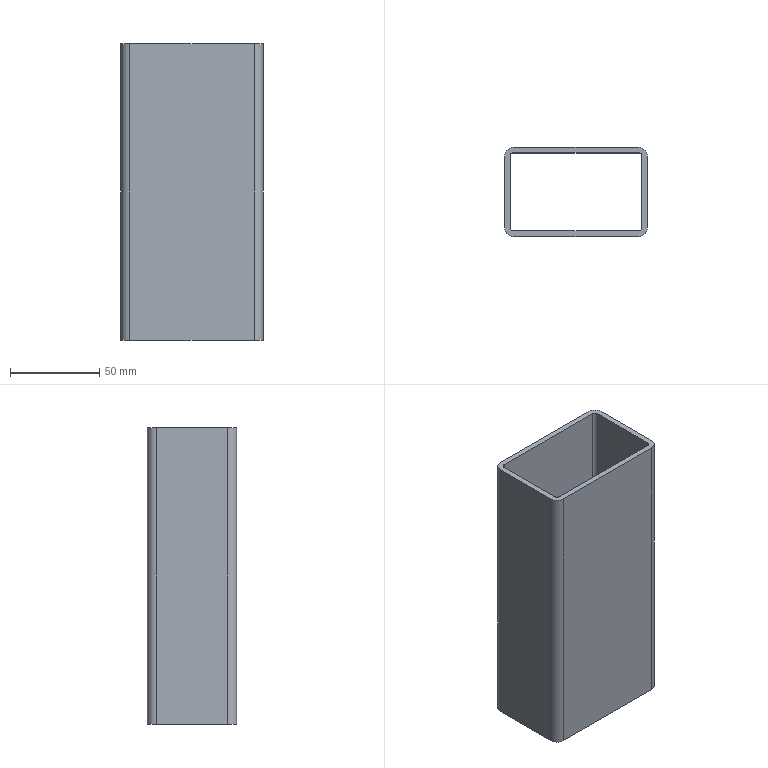Part | SolidWorks | features Extrusion 1, Fillet 1, Shell 1 | 1 solid | 18 faces | box 80 x 50 x 166 mm | volume 120512 mm3 | plane 10 | cylinder 8 | commonest cylinder face diameters 4 x4 10 x4
STEP:
#1=CARTESIAN_POINT('',(40.,-20.,0.));
#2=VERTEX_POINT('',#1);
#3=CARTESIAN_POINT('',(40.,20.,0.));
#4=VERTEX_POINT('',#3);
#5=CARTESIAN_POINT('',(40.,25.,0.));
#6=DIRECTION('',(0.,1.,0.));
#7=VECTOR('',#6,1000.);
#8=LINE('',#5,#7);
#9=EDGE_CURVE('',#2,#4,#8,.T.);
#10=ORIENTED_EDGE('',*,*,#9,.F.);
#11=CARTESIAN_POINT('',(35.,-25.,0.));
#12=VERTEX_POINT('',#11);
#13=CARTESIAN_POINT('',(35.,-20.,0.));
#14=DIRECTION('',(0.,0.,-1.));
#15=DIRECTION('',(-1.,0.,0.));
#16=AXIS2_PLACEMENT_3D('',#13,#14,#15);
#17=CIRCLE('',#16,5.);
#18=EDGE_CURVE('',#2,#12,#17,.T.);
#19=ORIENTED_EDGE('',*,*,#18,.T.);
#20=CARTESIAN_POINT('',(-35.,-25.,0.));
#21=VERTEX_POINT('',#20);
#22=CARTESIAN_POINT('',(40.,-25.,0.));
#23=DIRECTION('',(1.,0.,0.));
#24=VECTOR('',#23,1000.);
#25=LINE('',#22,#24);
#26=EDGE_CURVE('',#21,#12,#25,.T.);
#27=ORIENTED_EDGE('',*,*,#26,.F.);
#28=CARTESIAN_POINT('',(-40.,-20.,0.));
#29=VERTEX_POINT('',#28);
#30=CARTESIAN_POINT('',(-35.,-20.,0.));
#31=DIRECTION('',(0.,0.,-1.));
#32=DIRECTION('',(-1.,0.,0.));
#33=AXIS2_PLACEMENT_3D('',#30,#31,#32);
#34=CIRCLE('',#33,5.);
#35=EDGE_CURVE('',#21,#29,#34,.T.);
#36=ORIENTED_EDGE('',*,*,#35,.T.);
#37=CARTESIAN_POINT('',(-40.,20.,0.));
#38=VERTEX_POINT('',#37);
#39=CARTESIAN_POINT('',(-40.,25.,0.));
#40=DIRECTION('',(0.,-1.,0.));
#41=VECTOR('',#40,1000.);
#42=LINE('',#39,#41);
#43=EDGE_CURVE('',#38,#29,#42,.T.);
#44=ORIENTED_EDGE('',*,*,#43,.F.);
#45=CARTESIAN_POINT('',(-35.,25.,0.));
#46=VERTEX_POINT('',#45);
#47=CARTESIAN_POINT('',(-35.,20.,0.));
#48=DIRECTION('',(0.,0.,-1.));
#49=DIRECTION('',(-1.,0.,0.));
#50=AXIS2_PLACEMENT_3D('',#47,#48,#49);
#51=CIRCLE('',#50,5.);
#52=EDGE_CURVE('',#38,#46,#51,.T.);
#53=ORIENTED_EDGE('',*,*,#52,.T.);
#54=CARTESIAN_POINT('',(35.,25.,0.));
#55=VERTEX_POINT('',#54);
#56=CARTESIAN_POINT('',(40.,25.,0.));
#57=DIRECTION('',(-1.,0.,0.));
#58=VECTOR('',#57,1000.);
#59=LINE('',#56,#58);
#60=EDGE_CURVE('',#55,#46,#59,.T.);
#61=ORIENTED_EDGE('',*,*,#60,.F.);
#62=CARTESIAN_POINT('',(35.,20.,0.));
#63=DIRECTION('',(0.,0.,-1.));
#64=DIRECTION('',(-1.,0.,0.));
#65=AXIS2_PLACEMENT_3D('',#62,#63,#64);
#66=CIRCLE('',#65,5.);
#67=EDGE_CURVE('',#55,#4,#66,.T.);
#68=ORIENTED_EDGE('',*,*,#67,.T.);
#69=EDGE_LOOP('',(#10,#19,#27,#36,#44,#53,#61,#68));
#70=FACE_OUTER_BOUND('',#69,.T.);
#71=CARTESIAN_POINT('',(37.,-20.,0.));
#72=VERTEX_POINT('',#71);
#73=CARTESIAN_POINT('',(35.,-22.,0.));
#74=VERTEX_POINT('',#73);
#75=CARTESIAN_POINT('',(35.,-20.,0.));
#76=DIRECTION('',(0.,0.,-1.));
#77=DIRECTION('',(-1.,0.,0.));
#78=AXIS2_PLACEMENT_3D('',#75,#76,#77);
#79=CIRCLE('',#78,2.);
#80=EDGE_CURVE('',#72,#74,#79,.T.);
#81=ORIENTED_EDGE('',*,*,#80,.F.);
#82=CARTESIAN_POINT('',(37.,20.,0.));
#83=VERTEX_POINT('',#82);
#84=CARTESIAN_POINT('',(37.,0.,0.));
#85=DIRECTION('',(0.,1.,0.));
#86=VECTOR('',#85,1000.);
#87=LINE('',#84,#86);
#88=EDGE_CURVE('',#72,#83,#87,.T.);
#89=ORIENTED_EDGE('',*,*,#88,.T.);
#90=CARTESIAN_POINT('',(35.,22.,0.));
#91=VERTEX_POINT('',#90);
#92=CARTESIAN_POINT('',(35.,20.,0.));
#93=DIRECTION('',(0.,0.,-1.));
#94=DIRECTION('',(-1.,0.,0.));
#95=AXIS2_PLACEMENT_3D('',#92,#93,#94);
#96=CIRCLE('',#95,2.);
#97=EDGE_CURVE('',#91,#83,#96,.T.);
#98=ORIENTED_EDGE('',*,*,#97,.F.);
#99=CARTESIAN_POINT('',(-35.,22.,0.));
#100=VERTEX_POINT('',#99);
#101=CARTESIAN_POINT('',(0.,22.,0.));
#102=DIRECTION('',(-1.,0.,0.));
#103=VECTOR('',#102,1000.);
#104=LINE('',#101,#103);
#105=EDGE_CURVE('',#91,#100,#104,.T.);
#106=ORIENTED_EDGE('',*,*,#105,.T.);
#107=CARTESIAN_POINT('',(-37.,20.,0.));
#108=VERTEX_POINT('',#107);
#109=CARTESIAN_POINT('',(-35.,20.,0.));
#110=DIRECTION('',(0.,0.,-1.));
#111=DIRECTION('',(-1.,0.,0.));
#112=AXIS2_PLACEMENT_3D('',#109,#110,#111);
#113=CIRCLE('',#112,2.);
#114=EDGE_CURVE('',#108,#100,#113,.T.);
#115=ORIENTED_EDGE('',*,*,#114,.F.);
#116=CARTESIAN_POINT('',(-37.,-20.,0.));
#117=VERTEX_POINT('',#116);
#118=CARTESIAN_POINT('',(-37.,0.,0.));
#119=DIRECTION('',(0.,-1.,0.));
#120=VECTOR('',#119,1000.);
#121=LINE('',#118,#120);
#122=EDGE_CURVE('',#108,#117,#121,.T.);
#123=ORIENTED_EDGE('',*,*,#122,.T.);
#124=CARTESIAN_POINT('',(-35.,-22.,0.));
#125=VERTEX_POINT('',#124);
#126=CARTESIAN_POINT('',(-35.,-20.,0.));
#127=DIRECTION('',(0.,0.,-1.));
#128=DIRECTION('',(-1.,0.,0.));
#129=AXIS2_PLACEMENT_3D('',#126,#127,#128);
#130=CIRCLE('',#129,2.);
#131=EDGE_CURVE('',#125,#117,#130,.T.);
#132=ORIENTED_EDGE('',*,*,#131,.F.);
#133=CARTESIAN_POINT('',(0.,-22.,0.));
#134=DIRECTION('',(1.,0.,0.));
#135=VECTOR('',#134,1000.);
#136=LINE('',#133,#135);
#137=EDGE_CURVE('',#125,#74,#136,.T.);
#138=ORIENTED_EDGE('',*,*,#137,.T.);
#139=EDGE_LOOP('',(#81,#89,#98,#106,#115,#123,#132,#138));
#140=FACE_BOUND('',#139,.T.);
#141=CARTESIAN_POINT('',(0.,0.,0.));
#142=DIRECTION('',(0.,0.,-1.));
#143=DIRECTION('',(-1.,0.,0.));
#144=AXIS2_PLACEMENT_3D('',#141,#142,#143);
#145=PLANE('',#144);
#146=ADVANCED_FACE('',(#70,#140),#145,.T.);
#147=ORIENTED_EDGE('',*,*,#43,.T.);
#148=CARTESIAN_POINT('',(-40.,-20.,166.));
#149=VERTEX_POINT('',#148);
#150=CARTESIAN_POINT('',(-40.,-20.,166.));
#151=DIRECTION('',(0.,0.,1.));
#152=VECTOR('',#151,1000.);
#153=LINE('',#150,#152);
#154=EDGE_CURVE('',#29,#149,#153,.T.);
#155=ORIENTED_EDGE('',*,*,#154,.T.);
#156=CARTESIAN_POINT('',(-40.,20.,166.));
#157=VERTEX_POINT('',#156);
#158=CARTESIAN_POINT('',(-40.,25.,166.));
#159=DIRECTION('',(0.,-1.,0.));
#160=VECTOR('',#159,1000.);
#161=LINE('',#158,#160);
#162=EDGE_CURVE('',#157,#149,#161,.T.);
#163=ORIENTED_EDGE('',*,*,#162,.F.);
#164=CARTESIAN_POINT('',(-40.,20.,166.));
#165=DIRECTION('',(0.,0.,-1.));
#166=VECTOR('',#165,1000.);
#167=LINE('',#164,#166);
#168=EDGE_CURVE('',#157,#38,#167,.T.);
#169=ORIENTED_EDGE('',*,*,#168,.T.);
#170=EDGE_LOOP('',(#147,#155,#163,#169));
#171=FACE_OUTER_BOUND('',#170,.T.);
#172=CARTESIAN_POINT('',(-40.,25.,166.));
#173=DIRECTION('',(1.,0.,0.));
#174=DIRECTION('',(0.,0.,-1.));
#175=AXIS2_PLACEMENT_3D('',#172,#173,#174);
#176=PLANE('',#175);
#177=ADVANCED_FACE('',(#171),#176,.F.);
#178=ORIENTED_EDGE('',*,*,#26,.T.);
#179=CARTESIAN_POINT('',(35.,-25.,166.));
#180=VERTEX_POINT('',#179);
#181=CARTESIAN_POINT('',(35.,-25.,166.));
#182=DIRECTION('',(0.,0.,1.));
#183=VECTOR('',#182,1000.);
#184=LINE('',#181,#183);
#185=EDGE_CURVE('',#12,#180,#184,.T.);
#186=ORIENTED_EDGE('',*,*,#185,.T.);
#187=CARTESIAN_POINT('',(-35.,-25.,166.));
#188=VERTEX_POINT('',#187);
#189=CARTESIAN_POINT('',(40.,-25.,166.));
#190=DIRECTION('',(1.,0.,0.));
#191=VECTOR('',#190,1000.);
#192=LINE('',#189,#191);
#193=EDGE_CURVE('',#188,#180,#192,.T.);
#194=ORIENTED_EDGE('',*,*,#193,.F.);
#195=CARTESIAN_POINT('',(-35.,-25.,166.));
#196=DIRECTION('',(0.,0.,-1.));
#197=VECTOR('',#196,1000.);
#198=LINE('',#195,#197);
#199=EDGE_CURVE('',#188,#21,#198,.T.);
#200=ORIENTED_EDGE('',*,*,#199,.T.);
#201=EDGE_LOOP('',(#178,#186,#194,#200));
#202=FACE_OUTER_BOUND('',#201,.T.);
#203=CARTESIAN_POINT('',(40.,-25.,166.));
#204=DIRECTION('',(0.,1.,0.));
#205=DIRECTION('',(-1.,0.,0.));
#206=AXIS2_PLACEMENT_3D('',#203,#204,#205);
#207=PLANE('',#206);
#208=ADVANCED_FACE('',(#202),#207,.F.);
#209=CARTESIAN_POINT('',(40.,-20.,166.));
#210=VERTEX_POINT('',#209);
#211=CARTESIAN_POINT('',(40.,20.,166.));
#212=VERTEX_POINT('',#211);
#213=CARTESIAN_POINT('',(40.,25.,166.));
#214=DIRECTION('',(0.,1.,0.));
#215=VECTOR('',#214,1000.);
#216=LINE('',#213,#215);
#217=EDGE_CURVE('',#210,#212,#216,.T.);
#218=ORIENTED_EDGE('',*,*,#217,.F.);
#219=CARTESIAN_POINT('',(40.,-20.,166.));
#220=DIRECTION('',(0.,0.,-1.));
#221=VECTOR('',#220,1000.);
#222=LINE('',#219,#221);
#223=EDGE_CURVE('',#210,#2,#222,.T.);
#224=ORIENTED_EDGE('',*,*,#223,.T.);
#225=ORIENTED_EDGE('',*,*,#9,.T.);
#226=CARTESIAN_POINT('',(40.,20.,166.));
#227=DIRECTION('',(0.,0.,1.));
#228=VECTOR('',#227,1000.);
#229=LINE('',#226,#228);
#230=EDGE_CURVE('',#4,#212,#229,.T.);
#231=ORIENTED_EDGE('',*,*,#230,.T.);
#232=EDGE_LOOP('',(#218,#224,#225,#231));
#233=FACE_OUTER_BOUND('',#232,.T.);
#234=CARTESIAN_POINT('',(40.,25.,166.));
#235=DIRECTION('',(-1.,0.,0.));
#236=DIRECTION('',(0.,-1.,0.));
#237=AXIS2_PLACEMENT_3D('',#234,#235,#236);
#238=PLANE('',#237);
#239=ADVANCED_FACE('',(#233),#238,.F.);
#240=ORIENTED_EDGE('',*,*,#60,.T.);
#241=CARTESIAN_POINT('',(-35.,25.,166.));
#242=VERTEX_POINT('',#241);
#243=CARTESIAN_POINT('',(-35.,25.,166.));
#244=DIRECTION('',(0.,0.,1.));
#245=VECTOR('',#244,1000.);
#246=LINE('',#243,#245);
#247=EDGE_CURVE('',#46,#242,#246,.T.);
#248=ORIENTED_EDGE('',*,*,#247,.T.);
#249=CARTESIAN_POINT('',(35.,25.,166.));
#250=VERTEX_POINT('',#249);
#251=CARTESIAN_POINT('',(40.,25.,166.));
#252=DIRECTION('',(-1.,0.,0.));
#253=VECTOR('',#252,1000.);
#254=LINE('',#251,#253);
#255=EDGE_CURVE('',#250,#242,#254,.T.);
#256=ORIENTED_EDGE('',*,*,#255,.F.);
#257=CARTESIAN_POINT('',(35.,25.,166.));
#258=DIRECTION('',(0.,0.,-1.));
#259=VECTOR('',#258,1000.);
#260=LINE('',#257,#259);
#261=EDGE_CURVE('',#250,#55,#260,.T.);
#262=ORIENTED_EDGE('',*,*,#261,.T.);
#263=EDGE_LOOP('',(#240,#248,#256,#262));
#264=FACE_OUTER_BOUND('',#263,.T.);
#265=CARTESIAN_POINT('',(40.,25.,166.));
#266=DIRECTION('',(0.,-1.,0.));
#267=DIRECTION('',(1.,0.,0.));
#268=AXIS2_PLACEMENT_3D('',#265,#266,#267);
#269=PLANE('',#268);
#270=ADVANCED_FACE('',(#264),#269,.F.);
#271=CARTESIAN_POINT('',(-35.,-22.,166.));
#272=VERTEX_POINT('',#271);
#273=CARTESIAN_POINT('',(35.,-22.,166.));
#274=VERTEX_POINT('',#273);
#275=CARTESIAN_POINT('',(0.,-22.,166.));
#276=DIRECTION('',(1.,0.,0.));
#277=VECTOR('',#276,1000.);
#278=LINE('',#275,#277);
#279=EDGE_CURVE('',#272,#274,#278,.T.);
#280=ORIENTED_EDGE('',*,*,#279,.F.);
#281=CARTESIAN_POINT('',(-37.,-20.,166.));
#282=VERTEX_POINT('',#281);
#283=CARTESIAN_POINT('',(-35.,-20.,166.));
#284=DIRECTION('',(0.,0.,1.));
#285=DIRECTION('',(-1.,0.,0.));
#286=AXIS2_PLACEMENT_3D('',#283,#284,#285);
#287=CIRCLE('',#286,2.);
#288=EDGE_CURVE('',#282,#272,#287,.T.);
#289=ORIENTED_EDGE('',*,*,#288,.F.);
#290=CARTESIAN_POINT('',(-37.,20.,166.));
#291=VERTEX_POINT('',#290);
#292=CARTESIAN_POINT('',(-37.,0.,166.));
#293=DIRECTION('',(0.,-1.,0.));
#294=VECTOR('',#293,1000.);
#295=LINE('',#292,#294);
#296=EDGE_CURVE('',#291,#282,#295,.T.);
#297=ORIENTED_EDGE('',*,*,#296,.F.);
#298=CARTESIAN_POINT('',(-35.,22.,166.));
#299=VERTEX_POINT('',#298);
#300=CARTESIAN_POINT('',(-35.,20.,166.));
#301=DIRECTION('',(0.,0.,1.));
#302=DIRECTION('',(-1.,0.,0.));
#303=AXIS2_PLACEMENT_3D('',#300,#301,#302);
#304=CIRCLE('',#303,2.);
#305=EDGE_CURVE('',#299,#291,#304,.T.);
#306=ORIENTED_EDGE('',*,*,#305,.F.);
#307=CARTESIAN_POINT('',(35.,22.,166.));
#308=VERTEX_POINT('',#307);
#309=CARTESIAN_POINT('',(0.,22.,166.));
#310=DIRECTION('',(-1.,0.,0.));
#311=VECTOR('',#310,1000.);
#312=LINE('',#309,#311);
#313=EDGE_CURVE('',#308,#299,#312,.T.);
#314=ORIENTED_EDGE('',*,*,#313,.F.);
#315=CARTESIAN_POINT('',(37.,20.,166.));
#316=VERTEX_POINT('',#315);
#317=CARTESIAN_POINT('',(35.,20.,166.));
#318=DIRECTION('',(0.,0.,1.));
#319=DIRECTION('',(-1.,0.,0.));
#320=AXIS2_PLACEMENT_3D('',#317,#318,#319);
#321=CIRCLE('',#320,2.);
#322=EDGE_CURVE('',#316,#308,#321,.T.);
#323=ORIENTED_EDGE('',*,*,#322,.F.);
#324=CARTESIAN_POINT('',(37.,-20.,166.));
#325=VERTEX_POINT('',#324);
#326=CARTESIAN_POINT('',(37.,0.,166.));
#327=DIRECTION('',(0.,1.,0.));
#328=VECTOR('',#327,1000.);
#329=LINE('',#326,#328);
#330=EDGE_CURVE('',#325,#316,#329,.T.);
#331=ORIENTED_EDGE('',*,*,#330,.F.);
#332=CARTESIAN_POINT('',(35.,-20.,166.));
#333=DIRECTION('',(0.,0.,1.));
#334=DIRECTION('',(-1.,0.,0.));
#335=AXIS2_PLACEMENT_3D('',#332,#333,#334);
#336=CIRCLE('',#335,2.);
#337=EDGE_CURVE('',#274,#325,#336,.T.);
#338=ORIENTED_EDGE('',*,*,#337,.F.);
#339=EDGE_LOOP('',(#280,#289,#297,#306,#314,#323,#331,#338));
#340=FACE_BOUND('',#339,.T.);
#341=ORIENTED_EDGE('',*,*,#193,.T.);
#342=CARTESIAN_POINT('',(35.,-20.,166.));
#343=DIRECTION('',(0.,0.,1.));
#344=DIRECTION('',(-1.,0.,0.));
#345=AXIS2_PLACEMENT_3D('',#342,#343,#344);
#346=CIRCLE('',#345,5.);
#347=EDGE_CURVE('',#180,#210,#346,.T.);
#348=ORIENTED_EDGE('',*,*,#347,.T.);
#349=ORIENTED_EDGE('',*,*,#217,.T.);
#350=CARTESIAN_POINT('',(35.,20.,166.));
#351=DIRECTION('',(0.,0.,1.));
#352=DIRECTION('',(-1.,0.,0.));
#353=AXIS2_PLACEMENT_3D('',#350,#351,#352);
#354=CIRCLE('',#353,5.);
#355=EDGE_CURVE('',#212,#250,#354,.T.);
#356=ORIENTED_EDGE('',*,*,#355,.T.);
#357=ORIENTED_EDGE('',*,*,#255,.T.);
#358=CARTESIAN_POINT('',(-35.,20.,166.));
#359=DIRECTION('',(0.,0.,1.));
#360=DIRECTION('',(-1.,0.,0.));
#361=AXIS2_PLACEMENT_3D('',#358,#359,#360);
#362=CIRCLE('',#361,5.);
#363=EDGE_CURVE('',#242,#157,#362,.T.);
#364=ORIENTED_EDGE('',*,*,#363,.T.);
#365=ORIENTED_EDGE('',*,*,#162,.T.);
#366=CARTESIAN_POINT('',(-35.,-20.,166.));
#367=DIRECTION('',(0.,0.,1.));
#368=DIRECTION('',(-1.,0.,0.));
#369=AXIS2_PLACEMENT_3D('',#366,#367,#368);
#370=CIRCLE('',#369,5.);
#371=EDGE_CURVE('',#149,#188,#370,.T.);
#372=ORIENTED_EDGE('',*,*,#371,.T.);
#373=EDGE_LOOP('',(#341,#348,#349,#356,#357,#364,#365,#372));
#374=FACE_OUTER_BOUND('',#373,.T.);
#375=CARTESIAN_POINT('',(0.,0.,166.));
#376=DIRECTION('',(0.,0.,-1.));
#377=DIRECTION('',(-1.,0.,0.));
#378=AXIS2_PLACEMENT_3D('',#375,#376,#377);
#379=PLANE('',#378);
#380=ADVANCED_FACE('',(#340,#374),#379,.F.);
#381=ORIENTED_EDGE('',*,*,#347,.F.);
#382=ORIENTED_EDGE('',*,*,#185,.F.);
#383=ORIENTED_EDGE('',*,*,#18,.F.);
#384=ORIENTED_EDGE('',*,*,#223,.F.);
#385=EDGE_LOOP('',(#381,#382,#383,#384));
#386=FACE_OUTER_BOUND('',#385,.T.);
#387=CARTESIAN_POINT('',(35.,-20.,166.));
#388=DIRECTION('',(0.,0.,-1.));
#389=DIRECTION('',(-1.,0.,0.));
#390=AXIS2_PLACEMENT_3D('',#387,#388,#389);
#391=CYLINDRICAL_SURFACE('',#390,5.);
#392=ADVANCED_FACE('',(#386),#391,.T.);
#393=ORIENTED_EDGE('',*,*,#371,.F.);
#394=ORIENTED_EDGE('',*,*,#154,.F.);
#395=ORIENTED_EDGE('',*,*,#35,.F.);
#396=ORIENTED_EDGE('',*,*,#199,.F.);
#397=EDGE_LOOP('',(#393,#394,#395,#396));
#398=FACE_OUTER_BOUND('',#397,.T.);
#399=CARTESIAN_POINT('',(-35.,-20.,166.));
#400=DIRECTION('',(0.,0.,-1.));
#401=DIRECTION('',(-1.,0.,0.));
#402=AXIS2_PLACEMENT_3D('',#399,#400,#401);
#403=CYLINDRICAL_SURFACE('',#402,5.);
#404=ADVANCED_FACE('',(#398),#403,.T.);
#405=ORIENTED_EDGE('',*,*,#363,.F.);
#406=ORIENTED_EDGE('',*,*,#247,.F.);
#407=ORIENTED_EDGE('',*,*,#52,.F.);
#408=ORIENTED_EDGE('',*,*,#168,.F.);
#409=EDGE_LOOP('',(#405,#406,#407,#408));
#410=FACE_OUTER_BOUND('',#409,.T.);
#411=CARTESIAN_POINT('',(-35.,20.,166.));
#412=DIRECTION('',(0.,0.,-1.));
#413=DIRECTION('',(-1.,0.,0.));
#414=AXIS2_PLACEMENT_3D('',#411,#412,#413);
#415=CYLINDRICAL_SURFACE('',#414,5.);
#416=ADVANCED_FACE('',(#410),#415,.T.);
#417=ORIENTED_EDGE('',*,*,#355,.F.);
#418=ORIENTED_EDGE('',*,*,#230,.F.);
#419=ORIENTED_EDGE('',*,*,#67,.F.);
#420=ORIENTED_EDGE('',*,*,#261,.F.);
#421=EDGE_LOOP('',(#417,#418,#419,#420));
#422=FACE_OUTER_BOUND('',#421,.T.);
#423=CARTESIAN_POINT('',(35.,20.,166.));
#424=DIRECTION('',(0.,0.,-1.));
#425=DIRECTION('',(-1.,0.,0.));
#426=AXIS2_PLACEMENT_3D('',#423,#424,#425);
#427=CYLINDRICAL_SURFACE('',#426,5.);
#428=ADVANCED_FACE('',(#422),#427,.T.);
#429=ORIENTED_EDGE('',*,*,#122,.F.);
#430=CARTESIAN_POINT('',(-37.,20.,166.));
#431=DIRECTION('',(0.,0.,-1.));
#432=VECTOR('',#431,1000.);
#433=LINE('',#430,#432);
#434=EDGE_CURVE('',#291,#108,#433,.T.);
#435=ORIENTED_EDGE('',*,*,#434,.F.);
#436=ORIENTED_EDGE('',*,*,#296,.T.);
#437=CARTESIAN_POINT('',(-37.,-20.,166.));
#438=DIRECTION('',(0.,0.,1.));
#439=VECTOR('',#438,1000.);
#440=LINE('',#437,#439);
#441=EDGE_CURVE('',#117,#282,#440,.T.);
#442=ORIENTED_EDGE('',*,*,#441,.F.);
#443=EDGE_LOOP('',(#429,#435,#436,#442));
#444=FACE_OUTER_BOUND('',#443,.T.);
#445=CARTESIAN_POINT('',(-37.,25.,166.));
#446=DIRECTION('',(1.,0.,0.));
#447=DIRECTION('',(0.,0.,-1.));
#448=AXIS2_PLACEMENT_3D('',#445,#446,#447);
#449=PLANE('',#448);
#450=ADVANCED_FACE('',(#444),#449,.T.);
#451=ORIENTED_EDGE('',*,*,#137,.F.);
#452=CARTESIAN_POINT('',(-35.,-22.,166.));
#453=DIRECTION('',(0.,0.,-1.));
#454=VECTOR('',#453,1000.);
#455=LINE('',#452,#454);
#456=EDGE_CURVE('',#272,#125,#455,.T.);
#457=ORIENTED_EDGE('',*,*,#456,.F.);
#458=ORIENTED_EDGE('',*,*,#279,.T.);
#459=CARTESIAN_POINT('',(35.,-22.,166.));
#460=DIRECTION('',(0.,0.,1.));
#461=VECTOR('',#460,1000.);
#462=LINE('',#459,#461);
#463=EDGE_CURVE('',#74,#274,#462,.T.);
#464=ORIENTED_EDGE('',*,*,#463,.F.);
#465=EDGE_LOOP('',(#451,#457,#458,#464));
#466=FACE_OUTER_BOUND('',#465,.T.);
#467=CARTESIAN_POINT('',(40.,-22.,166.));
#468=DIRECTION('',(0.,1.,0.));
#469=DIRECTION('',(-1.,0.,0.));
#470=AXIS2_PLACEMENT_3D('',#467,#468,#469);
#471=PLANE('',#470);
#472=ADVANCED_FACE('',(#466),#471,.T.);
#473=ORIENTED_EDGE('',*,*,#330,.T.);
#474=CARTESIAN_POINT('',(37.,20.,166.));
#475=DIRECTION('',(0.,0.,1.));
#476=VECTOR('',#475,1000.);
#477=LINE('',#474,#476);
#478=EDGE_CURVE('',#83,#316,#477,.T.);
#479=ORIENTED_EDGE('',*,*,#478,.F.);
#480=ORIENTED_EDGE('',*,*,#88,.F.);
#481=CARTESIAN_POINT('',(37.,-20.,166.));
#482=DIRECTION('',(0.,0.,-1.));
#483=VECTOR('',#482,1000.);
#484=LINE('',#481,#483);
#485=EDGE_CURVE('',#325,#72,#484,.T.);
#486=ORIENTED_EDGE('',*,*,#485,.F.);
#487=EDGE_LOOP('',(#473,#479,#480,#486));
#488=FACE_OUTER_BOUND('',#487,.T.);
#489=CARTESIAN_POINT('',(37.,25.,166.));
#490=DIRECTION('',(-1.,0.,0.));
#491=DIRECTION('',(0.,-1.,0.));
#492=AXIS2_PLACEMENT_3D('',#489,#490,#491);
#493=PLANE('',#492);
#494=ADVANCED_FACE('',(#488),#493,.T.);
#495=ORIENTED_EDGE('',*,*,#105,.F.);
#496=CARTESIAN_POINT('',(35.,22.,166.));
#497=DIRECTION('',(0.,0.,-1.));
#498=VECTOR('',#497,1000.);
#499=LINE('',#496,#498);
#500=EDGE_CURVE('',#308,#91,#499,.T.);
#501=ORIENTED_EDGE('',*,*,#500,.F.);
#502=ORIENTED_EDGE('',*,*,#313,.T.);
#503=CARTESIAN_POINT('',(-35.,22.,166.));
#504=DIRECTION('',(0.,0.,1.));
#505=VECTOR('',#504,1000.);
#506=LINE('',#503,#505);
#507=EDGE_CURVE('',#100,#299,#506,.T.);
#508=ORIENTED_EDGE('',*,*,#507,.F.);
#509=EDGE_LOOP('',(#495,#501,#502,#508));
#510=FACE_OUTER_BOUND('',#509,.T.);
#511=CARTESIAN_POINT('',(40.,22.,166.));
#512=DIRECTION('',(0.,-1.,0.));
#513=DIRECTION('',(1.,0.,0.));
#514=AXIS2_PLACEMENT_3D('',#511,#512,#513);
#515=PLANE('',#514);
#516=ADVANCED_FACE('',(#510),#515,.T.);
#517=ORIENTED_EDGE('',*,*,#337,.T.);
#518=ORIENTED_EDGE('',*,*,#485,.T.);
#519=ORIENTED_EDGE('',*,*,#80,.T.);
#520=ORIENTED_EDGE('',*,*,#463,.T.);
#521=EDGE_LOOP('',(#517,#518,#519,#520));
#522=FACE_OUTER_BOUND('',#521,.T.);
#523=CARTESIAN_POINT('',(35.,-20.,166.));
#524=DIRECTION('',(0.,0.,-1.));
#525=DIRECTION('',(-1.,0.,0.));
#526=AXIS2_PLACEMENT_3D('',#523,#524,#525);
#527=CYLINDRICAL_SURFACE('',#526,2.);
#528=ADVANCED_FACE('',(#522),#527,.F.);
#529=ORIENTED_EDGE('',*,*,#288,.T.);
#530=ORIENTED_EDGE('',*,*,#456,.T.);
#531=ORIENTED_EDGE('',*,*,#131,.T.);
#532=ORIENTED_EDGE('',*,*,#441,.T.);
#533=EDGE_LOOP('',(#529,#530,#531,#532));
#534=FACE_OUTER_BOUND('',#533,.T.);
#535=CARTESIAN_POINT('',(-35.,-20.,166.));
#536=DIRECTION('',(0.,0.,-1.));
#537=DIRECTION('',(-1.,0.,0.));
#538=AXIS2_PLACEMENT_3D('',#535,#536,#537);
#539=CYLINDRICAL_SURFACE('',#538,2.);
#540=ADVANCED_FACE('',(#534),#539,.F.);
#541=ORIENTED_EDGE('',*,*,#305,.T.);
#542=ORIENTED_EDGE('',*,*,#434,.T.);
#543=ORIENTED_EDGE('',*,*,#114,.T.);
#544=ORIENTED_EDGE('',*,*,#507,.T.);
#545=EDGE_LOOP('',(#541,#542,#543,#544));
#546=FACE_OUTER_BOUND('',#545,.T.);
#547=CARTESIAN_POINT('',(-35.,20.,166.));
#548=DIRECTION('',(0.,0.,-1.));
#549=DIRECTION('',(-1.,0.,0.));
#550=AXIS2_PLACEMENT_3D('',#547,#548,#549);
#551=CYLINDRICAL_SURFACE('',#550,2.);
#552=ADVANCED_FACE('',(#546),#551,.F.);
#553=ORIENTED_EDGE('',*,*,#322,.T.);
#554=ORIENTED_EDGE('',*,*,#500,.T.);
#555=ORIENTED_EDGE('',*,*,#97,.T.);
#556=ORIENTED_EDGE('',*,*,#478,.T.);
#557=EDGE_LOOP('',(#553,#554,#555,#556));
#558=FACE_OUTER_BOUND('',#557,.T.);
#559=CARTESIAN_POINT('',(35.,20.,166.));
#560=DIRECTION('',(0.,0.,-1.));
#561=DIRECTION('',(-1.,0.,0.));
#562=AXIS2_PLACEMENT_3D('',#559,#560,#561);
#563=CYLINDRICAL_SURFACE('',#562,2.);
#564=ADVANCED_FACE('',(#558),#563,.F.);
#565=CLOSED_SHELL('',(#146,#177,#208,#239,#270,#380,#392,#404,#416,#428,#450,#472,#494,#516,#528,#540,#552,#564));
#566=MANIFOLD_SOLID_BREP('',#565);
#567=CARTESIAN_POINT('',(0.,0.,0.));
#568=DIRECTION('',(0.,0.,1.));
#569=DIRECTION('',(1.,0.,0.));
#570=AXIS2_PLACEMENT_3D('',#567,#568,#569);
#571=(LENGTH_UNIT()NAMED_UNIT(*)SI_UNIT(.MILLI.,.METRE.));
#572=UNCERTAINTY_MEASURE_WITH_UNIT(LENGTH_MEASURE(0.00001),#571,'','');
#573=(NAMED_UNIT(*)PLANE_ANGLE_UNIT()SI_UNIT($,.RADIAN.));
#574=(NAMED_UNIT(*)SI_UNIT($,.STERADIAN.)SOLID_ANGLE_UNIT());
#575=(GEOMETRIC_REPRESENTATION_CONTEXT(3)GLOBAL_UNCERTAINTY_ASSIGNED_CONTEXT((#572))GLOBAL_UNIT_ASSIGNED_CONTEXT((#571,#573,#574))REPRESENTATION_CONTEXT('',''));
#576=ADVANCED_BREP_SHAPE_REPRESENTATION('',(#566,#570),#575);